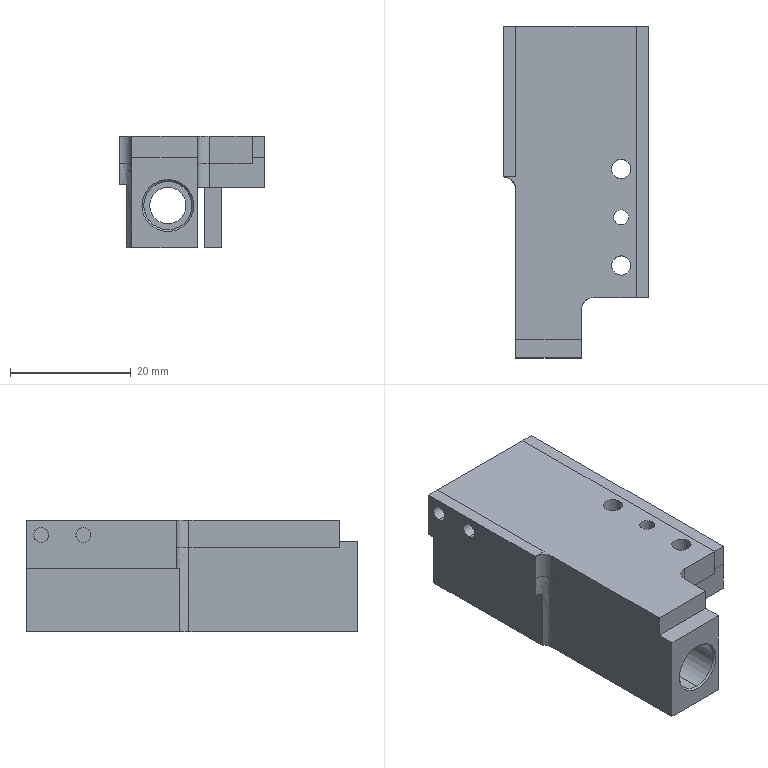NC program | NX | posted with a generic post | part box 24.15 x 55 x 18.5 mm
Whole program:
N10 G17 G21 G94 G90
(DRILLING_COPY_1_COPY_COPY , TOOL : D6A45)
N12 T07 M6
N14 G54
N16 G17 G0 G90 X11.5 Y-16.075 B0. C0. S5000 M3
N18 G43 Z30. H7
N20 G94 G81 G98 Z-1.6 F250. R3.
N22 G80
N24 G0 X11.5 Y-16.075 Z30.
N26 M5
(DRILLING_COPY_1_COPY_COPY_COPY , TOOL : 5.5ZT)
N28 T15 M6
N30 G54
N32 G17 G0 G90 X11.5 Y-16.075 B0. C0. S1500 M3
N34 G43 Z30. H15
N36 G94 G83 G98 Z-37.152 F120. Q2. R3.
N38 G80
N40 G0 X11.5 Y-16.075 Z30.
N42 M5
(HOLE_MILLING_1 , TOOL : D6)
N44 T06 M6
N46 G54
N48 G17 G0 G90 X11.5 Y-16.075 B0. C0. S9500 M3
N50 G43 Z30. H6
N52 Z0.703
N54 G94 G3 X11.95 Y-15.625 R0.45 F1500.
N56 X11.5 Y-15.175 R0.45
N58 X11.5 Y-15.175 Z0.303 I0. J-0.9
N60 X11.5 Y-15.175 Z-0.097 I0. J-0.9
N62 X11.5 Y-15.175 Z-0.497 I0. J-0.9
N64 X11.5 Y-15.175 Z-0.897 I0. J-0.9
N66 X11.5 Y-15.175 Z-1.297 I0. J-0.9
N68 X11.5 Y-15.175 Z-1.697 I0. J-0.9
N70 X11.5 Y-15.175 Z-2.097 I0. J-0.9
N72 X11.5 Y-15.175 Z-2.497 I0. J-0.9
N74 X11.5 Y-15.175 Z-2.897 I0. J-0.9
N76 X11.5 Y-15.175 Z-3.297 I0. J-0.9
N78 X11.5 Y-15.175 Z-3.697 I0. J-0.9
N80 X11.5 Y-15.175 Z-4.097 I0. J-0.9
N82 X11.5 Y-15.175 Z-4.497 I0. J-0.9
N84 X11.5 Y-15.175 Z-4.897 I0. J-0.9
N86 X11.5 Y-15.175 Z-5.297 I0. J-0.9
N88 X11.5 Y-15.175 Z-5.697 I0. J-0.9
N90 X11.5 Y-15.175 Z-6.097 I0. J-0.9
N92 X11.5 Y-15.175 Z-6.497 I0. J-0.9
N94 X11.5 Y-15.175 Z-6.897 I0. J-0.9
N96 X11.5 Y-15.175 Z-7.297 I0. J-0.9
N98 X11.5 Y-15.175 Z-7.697 I0. J-0.9
N100 X11.5 Y-15.175 Z-8.097 I0. J-0.9
N102 X11.5 Y-15.175 Z-8.497 I0. J-0.9
N104 X11.5 Y-15.175 Z-8.897 I0. J-0.9
N106 X11.5 Y-15.175 Z-9.297 I0. J-0.9
N108 X11.5 Y-15.175 Z-9.697 I0. J-0.9
N110 X12.399 Y-16.032 Z-10. R-0.9
N112 X11.457 Y-15.176 R0.9
N114 X12.399 Y-16.032 R-0.9
N116 X11.928 Y-15.604 R0.45
N118 X11.5 Y-16.075 R0.45
N120 G0 Z30.
N122 M5
(HOLE_MILLING_1_COPY , TOOL : D4)
N124 T04 M6
N126 G54
N128 G17 G0 G90 X11.5 Y-16.075 B0. C0. S9500 M3
N130 G43 Z30. H4
N132 Z-9.
N134 G94 G3 X11.95 Y-15.625 R0.45 F1500.
N136 X11.5 Y-15.175 R0.45
N138 X11.5 Y-15.175 Z-9.4 I0. J-0.9
N140 X11.5 Y-15.175 Z-9.8 I0. J-0.9
N142 X11.5 Y-15.175 Z-10.2 I0. J-0.9
N144 X11.5 Y-15.175 Z-10.6 I0. J-0.9
N146 X11.5 Y-15.175 Z-11. I0. J-0.9
N148 X11.5 Y-15.175 Z-11.4 I0. J-0.9
N150 X11.5 Y-15.175 Z-11.8 I0. J-0.9
N152 X11.5 Y-15.175 Z-12.2 I0. J-0.9
N154 X11.5 Y-15.175 Z-12.6 I0. J-0.9
N156 X11.5 Y-15.175 Z-13. I0. J-0.9
N158 X11.5 Y-15.175 Z-13.4 I0. J-0.9
N160 X11.5 Y-15.175 Z-13.8 I0. J-0.9
N162 X11.5 Y-15.175 Z-14.2 I0. J-0.9
N164 X11.5 Y-15.175 Z-14.6 I0. J-0.9
N166 X11.5 Y-15.175 Z-15. I0. J-0.9
N168 X11.5 Y-15.175 Z-15.4 I0. J-0.9
N170 X11.5 Y-15.175 Z-15.8 I0. J-0.9
N172 X11.5 Y-15.175 Z-16.2 I0. J-0.9
N174 X11.5 Y-15.175 Z-16.6 I0. J-0.9
N176 X11.5 Y-15.175 Z-17. I0. J-0.9
N178 X11.5 Y-15.175 Z-17.4 I0. J-0.9
N180 X11.5 Y-15.175 Z-17.8 I0. J-0.9
N182 X11.5 Y-15.175 Z-18.2 I0. J-0.9
N184 X11.5 Y-15.175 Z-18.6 I0. J-0.9
N186 X11.5 Y-15.175 Z-19. I0. J-0.9
N188 X11.5 Y-15.175 Z-19.4 I0. J-0.9
N190 X11.5 Y-15.175 Z-19.8 I0. J-0.9
N192 X11.5 Y-15.175 Z-20.2 I0. J-0.9
N194 X11.5 Y-15.175 Z-20.6 I0. J-0.9
N196 X11.5 Y-15.175 Z-21. I0. J-0.9
N198 X11.5 Y-15.175 Z-21.4 I0. J-0.9
N200 X11.5 Y-15.175 Z-21.8 I0. J-0.9
N202 X11.5 Y-15.175 Z-22.2 I0. J-0.9
N204 X11.5 Y-15.175 Z-22.6 I0. J-0.9
N206 X11.5 Y-15.175 Z-23. I0. J-0.9
N208 X11.5 Y-15.175 Z-23.4 I0. J-0.9
N210 X11.5 Y-15.175 Z-23.8 I0. J-0.9
N212 X11.5 Y-16.975 Z-24. I0. J-0.9
N214 X12.4 Y-16.075 R0.9
N216 X11.5 Y-16.975 R-0.9
N218 X11.95 Y-16.525 R0.45
N220 X11.5 Y-16.075 R0.45
N222 G0 Z30.
N224 M5
(PLANAR_MILL_COPY_COPY , TOOL : D6A45)
N226 T07 M6
N228 G54
N230 G17 G0 G90 X12.029 Y-14.043 B0. C0. S9500 M3
N232 G43 Z30. H7
N234 Z2.
N236 G94 G1 Z-1. F1250.
N238 X12.266 Y-13.132
N240 G3 X11.5 Y-12.775 R1.
N242 X8.2 Y-16.075 R3.3
N244 X11.5 Y-19.375 R3.3
N246 X14.8 Y-16.075 R3.3
N248 X11.5 Y-12.775 R3.3
N250 X10.734 Y-13.132 R1.
N252 G1 X10.971 Y-14.043
N254 Z2.
N256 G0 Z30.
N258 M5
(刀补6 , TOOL : D6)
N260 T06 M6
N262 G54
N264 G17 G0 G90 X11.5 Y-16.075 B0. C0. S9500 M3
N266 G43 Z30. H6
N268 Z0.703
N270 G41 G94 G1 X11.6 Y-16.071 F1200. D6
N272 G3 X11.5 Y-15.125 R0.478
N274 X11.5 Y-15.125 Z-1.297 I0. J-0.95
N276 X11.5 Y-15.125 Z-3.297 I0. J-0.95
N278 X11.5 Y-15.125 Z-5.297 I0. J-0.95
N280 X11.5 Y-15.125 Z-7.297 I0. J-0.95
N282 X11.5 Y-15.125 Z-9.297 I0. J-0.95
N284 X10.737 Y-16.641 Z-10. R0.95
N286 X12.066 Y-16.838 R0.95
N288 X10.737 Y-16.641 R-0.95
N290 X11.557 Y-16.157 R0.478
N292 G40
N294 G1 X11.5 Y-16.075
N296 G0 Z30.
N298 M5
(刀补4 , TOOL : D4)
N300 T04 M6
N302 G54
N304 G17 G0 G90 X11.5 Y-16.075 B0. C0. S9500 M3
N306 G43 Z30. H4
N308 Z-9.
N310 G41 G94 G1 X11.6 Y-16.071 F1200. D4
N312 G3 X11.5 Y-15.125 R0.478
N314 X11.5 Y-15.125 Z-11. I0. J-0.95
N316 X11.5 Y-15.125 Z-13. I0. J-0.95
N318 X11.5 Y-15.125 Z-15. I0. J-0.95
N320 X11.5 Y-15.125 Z-17. I0. J-0.95
N322 X11.5 Y-15.125 Z-19. I0. J-0.95
N324 X11.5 Y-15.125 Z-21. I0. J-0.95
N326 X11.5 Y-15.125 Z-23. I0. J-0.95
N328 X11.5 Y-17.025 Z-24. I0. J-0.95
N330 X12.45 Y-16.075 R0.95
N332 X11.5 Y-17.025 R-0.95
N334 X11.6 Y-16.079 R0.478
N336 G40
N338 G1 X11.5 Y-16.075
N340 G0 Z30.
N342 M5
N344 M2